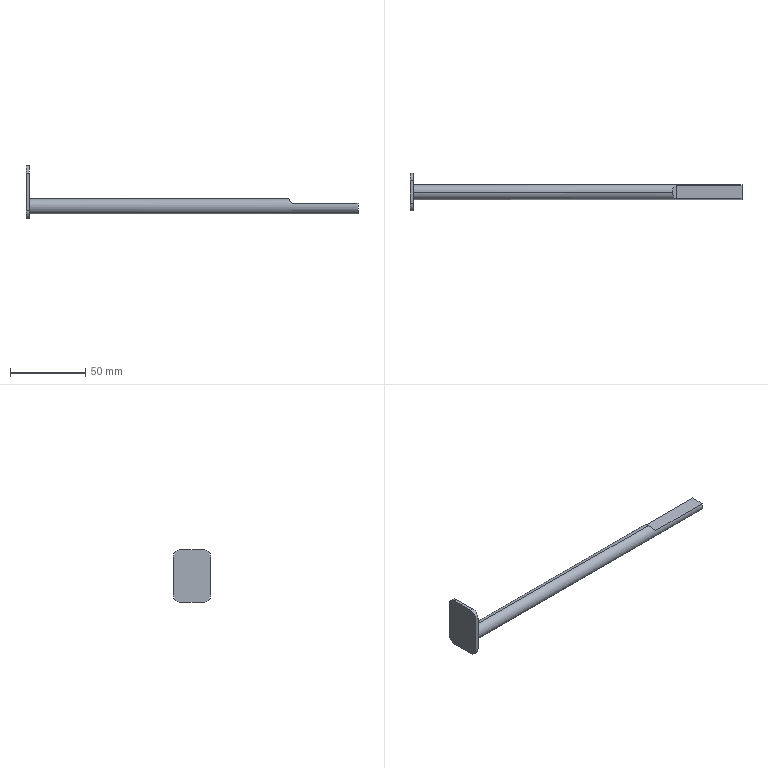Part | STEP file | 1 solid | 15 faces | box 220 x 25 x 35 mm | volume 17944 mm3 | plane 9 | cylinder 6 | commonest cylinder face diameters 10 x6
STEP:
#1=CARTESIAN_POINT('',(0.,0.,0.));
#2=DIRECTION('',(0.,0.,1.));
#3=DIRECTION('',(1.,0.,0.));
#4=AXIS2_PLACEMENT_3D('',#1,#2,#3);
#5=CARTESIAN_POINT('',(218.,45.399,13.874));
#6=VERTEX_POINT('',#5);
#7=CARTESIAN_POINT('',(218.,40.817,6.874));
#8=VERTEX_POINT('',#7);
#9=CARTESIAN_POINT('',(218.,40.817,11.874));
#10=DIRECTION('',(-1.,0.,0.));
#11=DIRECTION('',(0.,0.,1.));
#12=AXIS2_PLACEMENT_3D('',#9,#10,#11);
#13=CIRCLE('',#12,5.);
#14=CARTESIAN_POINT('',(218.,40.817,11.874));
#15=DIRECTION('',(-1.,0.,0.));
#16=DIRECTION('',(0.,0.,1.));
#17=AXIS2_PLACEMENT_3D('',#14,#15,#16);
#18=CYLINDRICAL_SURFACE('',#17,5.);
#19=CARTESIAN_POINT('',(0.,0.));
#20=DIRECTION('',(1.,0.));
#21=VECTOR('',#20,1.);
#22=LINE('',#19,#21);
#23=(GEOMETRIC_REPRESENTATION_CONTEXT(2)PARAMETRIC_REPRESENTATION_CONTEXT()REPRESENTATION_CONTEXT('',''));
#24=DEFINITIONAL_REPRESENTATION('',(#22),#23);
#25=PCURVE('',#18,#24);
#26=CARTESIAN_POINT('',(218.,40.817,11.874));
#27=DIRECTION('',(-1.,0.,0.));
#28=DIRECTION('',(0.,0.,1.));
#29=AXIS2_PLACEMENT_3D('',#26,#27,#28);
#30=PLANE('',#29);
#31=CARTESIAN_POINT('',(0.,0.));
#32=DIRECTION('',(1.,0.));
#33=AXIS2_PLACEMENT_2D('',#31,#32);
#34=CIRCLE('',#33,5.);
#35=(GEOMETRIC_REPRESENTATION_CONTEXT(2)PARAMETRIC_REPRESENTATION_CONTEXT()REPRESENTATION_CONTEXT('',''));
#36=DEFINITIONAL_REPRESENTATION('',(#34),#35);
#37=PCURVE('',#30,#36);
#38=SURFACE_CURVE('',#13,(#25,#37),.PCURVE_S1.);
#39=EDGE_CURVE('',#6,#8,#38,.T.);
#40=ORIENTED_EDGE('',*,*,#39,.T.);
#41=CARTESIAN_POINT('',(0.,40.817,6.874));
#42=VERTEX_POINT('',#41);
#43=CARTESIAN_POINT('',(218.,40.817,6.874));
#44=DIRECTION('',(-1.,0.,0.));
#45=VECTOR('',#44,1.);
#46=LINE('',#43,#45);
#47=CARTESIAN_POINT('',(3.142,0.));
#48=DIRECTION('',(0.,1.));
#49=VECTOR('',#48,1.);
#50=LINE('',#47,#49);
#51=(GEOMETRIC_REPRESENTATION_CONTEXT(2)PARAMETRIC_REPRESENTATION_CONTEXT()REPRESENTATION_CONTEXT('',''));
#52=DEFINITIONAL_REPRESENTATION('',(#50),#51);
#53=PCURVE('',#18,#52);
#54=CARTESIAN_POINT('',(218.,40.817,11.874));
#55=DIRECTION('',(-1.,0.,0.));
#56=DIRECTION('',(0.,0.,1.));
#57=AXIS2_PLACEMENT_3D('',#54,#55,#56);
#58=CYLINDRICAL_SURFACE('',#57,5.);
#59=CARTESIAN_POINT('',(3.142,0.));
#60=DIRECTION('',(0.,1.));
#61=VECTOR('',#60,1.);
#62=LINE('',#59,#61);
#63=(GEOMETRIC_REPRESENTATION_CONTEXT(2)PARAMETRIC_REPRESENTATION_CONTEXT()REPRESENTATION_CONTEXT('',''));
#64=DEFINITIONAL_REPRESENTATION('',(#62),#63);
#65=PCURVE('',#58,#64);
#66=SURFACE_CURVE('',#46,(#53,#65),.PCURVE_S1.);
#67=EDGE_CURVE('',#8,#42,#66,.T.);
#68=ORIENTED_EDGE('',*,*,#67,.T.);
#69=CARTESIAN_POINT('',(0.,40.817,16.874));
#70=VERTEX_POINT('',#69);
#71=CARTESIAN_POINT('',(0.,40.817,11.874));
#72=DIRECTION('',(1.,0.,0.));
#73=DIRECTION('',(0.,0.,-1.));
#74=AXIS2_PLACEMENT_3D('',#71,#72,#73);
#75=CIRCLE('',#74,5.);
#76=CARTESIAN_POINT('',(3.142,218.));
#77=DIRECTION('',(-1.,0.));
#78=VECTOR('',#77,1.);
#79=LINE('',#76,#78);
#80=(GEOMETRIC_REPRESENTATION_CONTEXT(2)PARAMETRIC_REPRESENTATION_CONTEXT()REPRESENTATION_CONTEXT('',''));
#81=DEFINITIONAL_REPRESENTATION('',(#79),#80);
#82=PCURVE('',#18,#81);
#83=CARTESIAN_POINT('',(0.,0.,0.));
#84=DIRECTION('',(1.,0.,0.));
#85=DIRECTION('',(0.,0.,-1.));
#86=AXIS2_PLACEMENT_3D('',#83,#84,#85);
#87=PLANE('',#86);
#88=CARTESIAN_POINT('',(-11.874,40.817));
#89=DIRECTION('',(1.,0.));
#90=AXIS2_PLACEMENT_2D('',#88,#89);
#91=CIRCLE('',#90,5.);
#92=(GEOMETRIC_REPRESENTATION_CONTEXT(2)PARAMETRIC_REPRESENTATION_CONTEXT()REPRESENTATION_CONTEXT('',''));
#93=DEFINITIONAL_REPRESENTATION('',(#91),#92);
#94=PCURVE('',#87,#93);
#95=SURFACE_CURVE('',#75,(#82,#94),.PCURVE_S1.);
#96=EDGE_CURVE('',#42,#70,#95,.T.);
#97=ORIENTED_EDGE('',*,*,#96,.T.);
#98=CARTESIAN_POINT('',(171.771,40.817,16.874));
#99=VERTEX_POINT('',#98);
#100=CARTESIAN_POINT('',(218.,40.817,16.874));
#101=DIRECTION('',(-1.,0.,0.));
#102=VECTOR('',#101,1.);
#103=LINE('',#100,#102);
#104=CARTESIAN_POINT('',(0.,0.));
#105=DIRECTION('',(0.,1.));
#106=VECTOR('',#105,1.);
#107=LINE('',#104,#106);
#108=(GEOMETRIC_REPRESENTATION_CONTEXT(2)PARAMETRIC_REPRESENTATION_CONTEXT()REPRESENTATION_CONTEXT('',''));
#109=DEFINITIONAL_REPRESENTATION('',(#107),#108);
#110=PCURVE('',#18,#109);
#111=CARTESIAN_POINT('',(6.283,0.));
#112=DIRECTION('',(0.,1.));
#113=VECTOR('',#112,1.);
#114=LINE('',#111,#113);
#115=(GEOMETRIC_REPRESENTATION_CONTEXT(2)PARAMETRIC_REPRESENTATION_CONTEXT()REPRESENTATION_CONTEXT('',''));
#116=DEFINITIONAL_REPRESENTATION('',(#114),#115);
#117=PCURVE('',#58,#116);
#118=SURFACE_CURVE('',#103,(#110,#117),.PCURVE_S1.);
#119=EDGE_CURVE('',#99,#70,#118,.T.);
#120=ORIENTED_EDGE('',*,*,#119,.F.);
#121=CARTESIAN_POINT('',(174.5,45.399,13.874));
#122=VERTEX_POINT('',#121);
#123=CARTESIAN_POINT('',(174.5,45.399,13.874));
#124=CARTESIAN_POINT('',(172.792,44.58,15.752));
#125=CARTESIAN_POINT('',(171.771,42.866,16.874));
#126=CARTESIAN_POINT('',(171.771,40.817,16.874));
#127=(BOUNDED_CURVE()B_SPLINE_CURVE(3,(#123,#124,#125,#126),.UNSPECIFIED.,.F.,.F.)B_SPLINE_CURVE_WITH_KNOTS((4,4),(5.124,6.283),.PIECEWISE_BEZIER_KNOTS.)CURVE()GEOMETRIC_REPRESENTATION_ITEM()RATIONAL_B_SPLINE_CURVE((1.,0.8911,0.8911,1.))REPRESENTATION_ITEM(''));
#128=CARTESIAN_POINT('',(1.159,43.5));
#129=CARTESIAN_POINT('',(1.143,43.569));
#130=CARTESIAN_POINT('',(1.109,43.707));
#131=CARTESIAN_POINT('',(1.058,43.912));
#132=CARTESIAN_POINT('',(1.007,44.113));
#133=CARTESIAN_POINT('',(0.9548,44.31));
#134=CARTESIAN_POINT('',(0.9022,44.501));
#135=CARTESIAN_POINT('',(0.8492,44.687));
#136=CARTESIAN_POINT('',(0.7957,44.865));
#137=CARTESIAN_POINT('',(0.742,45.035));
#138=CARTESIAN_POINT('',(0.688,45.196));
#139=CARTESIAN_POINT('',(0.6339,45.347));
#140=CARTESIAN_POINT('',(0.5796,45.488));
#141=CARTESIAN_POINT('',(0.5254,45.617));
#142=CARTESIAN_POINT('',(0.4713,45.735));
#143=CARTESIAN_POINT('',(0.4173,45.841));
#144=CARTESIAN_POINT('',(0.3635,45.934));
#145=CARTESIAN_POINT('',(0.3101,46.014));
#146=CARTESIAN_POINT('',(0.2571,46.081));
#147=CARTESIAN_POINT('',(0.2045,46.136));
#148=CARTESIAN_POINT('',(0.1524,46.178));
#149=CARTESIAN_POINT('',(0.1009,46.208));
#150=CARTESIAN_POINT('',(0.05004,46.225));
#151=CARTESIAN_POINT('',(0.0166,46.229));
#152=CARTESIAN_POINT('',(0.,46.229));
#153=B_SPLINE_CURVE_WITH_KNOTS('',3,(#128,#129,#130,#131,#132,#133,#134,#135,#136,#137,#138,#139,#140,#141,#142,#143,#144,#145,#146,#147,#148,#149,#150,#151,#152),.UNSPECIFIED.,.F.,.F.,(4,1,1,1,1,1,1,1,1,1,1,1,1,1,1,1,1,1,1,1,1,1,4),(5.124,5.177,5.229,5.282,5.335,5.387,5.44,5.493,5.545,5.598,5.651,5.704,5.756,5.809,5.862,5.914,5.967,6.02,6.072,6.125,6.178,6.23,6.283),.QUASI_UNIFORM_KNOTS.);
#154=(GEOMETRIC_REPRESENTATION_CONTEXT(2)PARAMETRIC_REPRESENTATION_CONTEXT()REPRESENTATION_CONTEXT('',''));
#155=DEFINITIONAL_REPRESENTATION('',(#153),#154);
#156=PCURVE('',#18,#155);
#157=CARTESIAN_POINT('',(174.5,53.317,13.874));
#158=DIRECTION('',(-0.7398,0.,-0.6729));
#159=DIRECTION('',(-0.6729,0.,0.7398));
#160=AXIS2_PLACEMENT_3D('',#157,#158,#159);
#161=PLANE('',#160);
#162=CARTESIAN_POINT('',(0.,-7.917));
#163=CARTESIAN_POINT('',(2.538,-8.737));
#164=CARTESIAN_POINT('',(4.055,-10.451));
#165=CARTESIAN_POINT('',(4.055,-12.5));
#166=(BOUNDED_CURVE()B_SPLINE_CURVE(3,(#162,#163,#164,#165),.UNSPECIFIED.,.F.,.F.)B_SPLINE_CURVE_WITH_KNOTS((4,4),(5.124,6.283),.PIECEWISE_BEZIER_KNOTS.)CURVE()GEOMETRIC_REPRESENTATION_ITEM()RATIONAL_B_SPLINE_CURVE((1.,0.8911,0.8911,1.))REPRESENTATION_ITEM(''));
#167=(GEOMETRIC_REPRESENTATION_CONTEXT(2)PARAMETRIC_REPRESENTATION_CONTEXT()REPRESENTATION_CONTEXT('',''));
#168=DEFINITIONAL_REPRESENTATION('',(#166),#167);
#169=PCURVE('',#161,#168);
#170=SURFACE_CURVE('',#127,(#156,#169),.PCURVE_S1.);
#171=EDGE_CURVE('',#122,#99,#170,.T.);
#172=ORIENTED_EDGE('',*,*,#171,.F.);
#173=CARTESIAN_POINT('',(218.,45.399,13.874));
#174=DIRECTION('',(-1.,0.,0.));
#175=VECTOR('',#174,1.);
#176=LINE('',#173,#175);
#177=CARTESIAN_POINT('',(1.159,0.));
#178=DIRECTION('',(0.,1.));
#179=VECTOR('',#178,1.);
#180=LINE('',#177,#179);
#181=(GEOMETRIC_REPRESENTATION_CONTEXT(2)PARAMETRIC_REPRESENTATION_CONTEXT()REPRESENTATION_CONTEXT('',''));
#182=DEFINITIONAL_REPRESENTATION('',(#180),#181);
#183=PCURVE('',#18,#182);
#184=CARTESIAN_POINT('',(174.5,21.274,13.874));
#185=DIRECTION('',(0.,0.,-1.));
#186=DIRECTION('',(-1.,0.,0.));
#187=AXIS2_PLACEMENT_3D('',#184,#185,#186);
#188=PLANE('',#187);
#189=CARTESIAN_POINT('',(-43.5,24.125));
#190=DIRECTION('',(1.,0.));
#191=VECTOR('',#190,1.);
#192=LINE('',#189,#191);
#193=(GEOMETRIC_REPRESENTATION_CONTEXT(2)PARAMETRIC_REPRESENTATION_CONTEXT()REPRESENTATION_CONTEXT('',''));
#194=DEFINITIONAL_REPRESENTATION('',(#192),#193);
#195=PCURVE('',#188,#194);
#196=SURFACE_CURVE('',#176,(#183,#195),.PCURVE_S1.);
#197=EDGE_CURVE('',#6,#122,#196,.T.);
#198=ORIENTED_EDGE('',*,*,#197,.F.);
#199=EDGE_LOOP('',(#40,#68,#97,#120,#172,#198));
#200=FACE_BOUND('',#199,.T.);
#201=ADVANCED_FACE('',(#200),#18,.T.);
#202=CARTESIAN_POINT('',(-2.,48.317,38.874));
#203=VERTEX_POINT('',#202);
#204=CARTESIAN_POINT('',(-2.,33.317,38.874));
#205=VERTEX_POINT('',#204);
#206=CARTESIAN_POINT('',(-2.,53.317,38.874));
#207=DIRECTION('',(0.,-1.,0.));
#208=VECTOR('',#207,1.);
#209=LINE('',#206,#208);
#210=CARTESIAN_POINT('',(-2.,53.317,38.874));
#211=DIRECTION('',(0.,0.,1.));
#212=DIRECTION('',(1.,0.,0.));
#213=AXIS2_PLACEMENT_3D('',#210,#211,#212);
#214=PLANE('',#213);
#215=CARTESIAN_POINT('',(0.,0.));
#216=DIRECTION('',(0.,-1.));
#217=VECTOR('',#216,1.);
#218=LINE('',#215,#217);
#219=(GEOMETRIC_REPRESENTATION_CONTEXT(2)PARAMETRIC_REPRESENTATION_CONTEXT()REPRESENTATION_CONTEXT('',''));
#220=DEFINITIONAL_REPRESENTATION('',(#218),#219);
#221=PCURVE('',#214,#220);
#222=CARTESIAN_POINT('',(-2.,0.,0.));
#223=DIRECTION('',(1.,0.,0.));
#224=DIRECTION('',(0.,0.,-1.));
#225=AXIS2_PLACEMENT_3D('',#222,#223,#224);
#226=PLANE('',#225);
#227=CARTESIAN_POINT('',(-38.874,53.317));
#228=DIRECTION('',(0.,-1.));
#229=VECTOR('',#228,1.);
#230=LINE('',#227,#229);
#231=(GEOMETRIC_REPRESENTATION_CONTEXT(2)PARAMETRIC_REPRESENTATION_CONTEXT()REPRESENTATION_CONTEXT('',''));
#232=DEFINITIONAL_REPRESENTATION('',(#230),#231);
#233=PCURVE('',#226,#232);
#234=SURFACE_CURVE('',#209,(#221,#233),.PCURVE_S1.);
#235=EDGE_CURVE('',#203,#205,#234,.T.);
#236=ORIENTED_EDGE('',*,*,#235,.T.);
#237=CARTESIAN_POINT('',(0.,33.317,38.874));
#238=VERTEX_POINT('',#237);
#239=CARTESIAN_POINT('',(-2.,33.317,38.874));
#240=DIRECTION('',(1.,0.,0.));
#241=VECTOR('',#240,1.);
#242=LINE('',#239,#241);
#243=CARTESIAN_POINT('',(0.,-20.));
#244=DIRECTION('',(1.,0.));
#245=VECTOR('',#244,1.);
#246=LINE('',#243,#245);
#247=(GEOMETRIC_REPRESENTATION_CONTEXT(2)PARAMETRIC_REPRESENTATION_CONTEXT()REPRESENTATION_CONTEXT('',''));
#248=DEFINITIONAL_REPRESENTATION('',(#246),#247);
#249=PCURVE('',#214,#248);
#250=CARTESIAN_POINT('',(-2.,33.317,33.874));
#251=DIRECTION('',(1.,0.,0.));
#252=DIRECTION('',(0.,0.,-1.));
#253=AXIS2_PLACEMENT_3D('',#250,#251,#252);
#254=CYLINDRICAL_SURFACE('',#253,5.);
#255=CARTESIAN_POINT('',(3.142,0.));
#256=DIRECTION('',(0.,1.));
#257=VECTOR('',#256,1.);
#258=LINE('',#255,#257);
#259=(GEOMETRIC_REPRESENTATION_CONTEXT(2)PARAMETRIC_REPRESENTATION_CONTEXT()REPRESENTATION_CONTEXT('',''));
#260=DEFINITIONAL_REPRESENTATION('',(#258),#259);
#261=PCURVE('',#254,#260);
#262=SURFACE_CURVE('',#242,(#249,#261),.PCURVE_S1.);
#263=EDGE_CURVE('',#205,#238,#262,.T.);
#264=ORIENTED_EDGE('',*,*,#263,.T.);
#265=CARTESIAN_POINT('',(0.,48.317,38.874));
#266=VERTEX_POINT('',#265);
#267=CARTESIAN_POINT('',(0.,53.317,38.874));
#268=DIRECTION('',(0.,-1.,0.));
#269=VECTOR('',#268,1.);
#270=LINE('',#267,#269);
#271=CARTESIAN_POINT('',(2.,0.));
#272=DIRECTION('',(0.,-1.));
#273=VECTOR('',#272,1.);
#274=LINE('',#271,#273);
#275=(GEOMETRIC_REPRESENTATION_CONTEXT(2)PARAMETRIC_REPRESENTATION_CONTEXT()REPRESENTATION_CONTEXT('',''));
#276=DEFINITIONAL_REPRESENTATION('',(#274),#275);
#277=PCURVE('',#214,#276);
#278=CARTESIAN_POINT('',(-38.874,53.317));
#279=DIRECTION('',(0.,-1.));
#280=VECTOR('',#279,1.);
#281=LINE('',#278,#280);
#282=(GEOMETRIC_REPRESENTATION_CONTEXT(2)PARAMETRIC_REPRESENTATION_CONTEXT()REPRESENTATION_CONTEXT('',''));
#283=DEFINITIONAL_REPRESENTATION('',(#281),#282);
#284=PCURVE('',#87,#283);
#285=SURFACE_CURVE('',#270,(#277,#284),.PCURVE_S1.);
#286=EDGE_CURVE('',#266,#238,#285,.T.);
#287=ORIENTED_EDGE('',*,*,#286,.F.);
#288=CARTESIAN_POINT('',(-2.,48.317,38.874));
#289=DIRECTION('',(-1.,0.,0.));
#290=VECTOR('',#289,1.);
#291=LINE('',#288,#290);
#292=CARTESIAN_POINT('',(0.,-5.));
#293=DIRECTION('',(-1.,0.));
#294=VECTOR('',#293,1.);
#295=LINE('',#292,#294);
#296=(GEOMETRIC_REPRESENTATION_CONTEXT(2)PARAMETRIC_REPRESENTATION_CONTEXT()REPRESENTATION_CONTEXT('',''));
#297=DEFINITIONAL_REPRESENTATION('',(#295),#296);
#298=PCURVE('',#214,#297);
#299=CARTESIAN_POINT('',(-2.,48.317,33.874));
#300=DIRECTION('',(1.,0.,0.));
#301=DIRECTION('',(0.,0.,-1.));
#302=AXIS2_PLACEMENT_3D('',#299,#300,#301);
#303=CYLINDRICAL_SURFACE('',#302,5.);
#304=CARTESIAN_POINT('',(3.142,0.));
#305=DIRECTION('',(0.,-1.));
#306=VECTOR('',#305,1.);
#307=LINE('',#304,#306);
#308=(GEOMETRIC_REPRESENTATION_CONTEXT(2)PARAMETRIC_REPRESENTATION_CONTEXT()REPRESENTATION_CONTEXT('',''));
#309=DEFINITIONAL_REPRESENTATION('',(#307),#308);
#310=PCURVE('',#303,#309);
#311=SURFACE_CURVE('',#291,(#298,#310),.PCURVE_S1.);
#312=EDGE_CURVE('',#266,#203,#311,.T.);
#313=ORIENTED_EDGE('',*,*,#312,.T.);
#314=EDGE_LOOP('',(#236,#264,#287,#313));
#315=FACE_BOUND('',#314,.T.);
#316=ADVANCED_FACE('',(#315),#214,.T.);
#317=CARTESIAN_POINT('',(0.,53.317,8.874));
#318=VERTEX_POINT('',#317);
#319=CARTESIAN_POINT('',(0.,53.317,33.874));
#320=VERTEX_POINT('',#319);
#321=CARTESIAN_POINT('',(0.,53.317,38.874));
#322=DIRECTION('',(0.,0.,1.));
#323=VECTOR('',#322,1.);
#324=LINE('',#321,#323);
#325=CARTESIAN_POINT('',(-2.,53.317,38.874));
#326=DIRECTION('',(0.,1.,0.));
#327=DIRECTION('',(0.,0.,1.));
#328=AXIS2_PLACEMENT_3D('',#325,#326,#327);
#329=PLANE('',#328);
#330=CARTESIAN_POINT('',(0.,2.));
#331=DIRECTION('',(1.,0.));
#332=VECTOR('',#331,1.);
#333=LINE('',#330,#332);
#334=(GEOMETRIC_REPRESENTATION_CONTEXT(2)PARAMETRIC_REPRESENTATION_CONTEXT()REPRESENTATION_CONTEXT('',''));
#335=DEFINITIONAL_REPRESENTATION('',(#333),#334);
#336=PCURVE('',#329,#335);
#337=CARTESIAN_POINT('',(-38.874,53.317));
#338=DIRECTION('',(-1.,0.));
#339=VECTOR('',#338,1.);
#340=LINE('',#337,#339);
#341=(GEOMETRIC_REPRESENTATION_CONTEXT(2)PARAMETRIC_REPRESENTATION_CONTEXT()REPRESENTATION_CONTEXT('',''));
#342=DEFINITIONAL_REPRESENTATION('',(#340),#341);
#343=PCURVE('',#87,#342);
#344=SURFACE_CURVE('',#324,(#336,#343),.PCURVE_S1.);
#345=EDGE_CURVE('',#318,#320,#344,.T.);
#346=ORIENTED_EDGE('',*,*,#345,.F.);
#347=CARTESIAN_POINT('',(-2.,53.317,8.874));
#348=VERTEX_POINT('',#347);
#349=CARTESIAN_POINT('',(-2.,53.317,8.874));
#350=DIRECTION('',(-1.,0.,0.));
#351=VECTOR('',#350,1.);
#352=LINE('',#349,#351);
#353=CARTESIAN_POINT('',(-30.,0.));
#354=DIRECTION('',(0.,-1.));
#355=VECTOR('',#354,1.);
#356=LINE('',#353,#355);
#357=(GEOMETRIC_REPRESENTATION_CONTEXT(2)PARAMETRIC_REPRESENTATION_CONTEXT()REPRESENTATION_CONTEXT('',''));
#358=DEFINITIONAL_REPRESENTATION('',(#356),#357);
#359=PCURVE('',#329,#358);
#360=CARTESIAN_POINT('',(-2.,48.317,8.874));
#361=DIRECTION('',(1.,0.,0.));
#362=DIRECTION('',(0.,0.,-1.));
#363=AXIS2_PLACEMENT_3D('',#360,#361,#362);
#364=CYLINDRICAL_SURFACE('',#363,5.);
#365=CARTESIAN_POINT('',(1.571,0.));
#366=DIRECTION('',(0.,-1.));
#367=VECTOR('',#366,1.);
#368=LINE('',#365,#367);
#369=(GEOMETRIC_REPRESENTATION_CONTEXT(2)PARAMETRIC_REPRESENTATION_CONTEXT()REPRESENTATION_CONTEXT('',''));
#370=DEFINITIONAL_REPRESENTATION('',(#368),#369);
#371=PCURVE('',#364,#370);
#372=SURFACE_CURVE('',#352,(#359,#371),.PCURVE_S1.);
#373=EDGE_CURVE('',#318,#348,#372,.T.);
#374=ORIENTED_EDGE('',*,*,#373,.T.);
#375=CARTESIAN_POINT('',(-2.,53.317,33.874));
#376=VERTEX_POINT('',#375);
#377=CARTESIAN_POINT('',(-2.,53.317,38.874));
#378=DIRECTION('',(0.,0.,1.));
#379=VECTOR('',#378,1.);
#380=LINE('',#377,#379);
#381=CARTESIAN_POINT('',(0.,0.));
#382=DIRECTION('',(1.,0.));
#383=VECTOR('',#382,1.);
#384=LINE('',#381,#383);
#385=(GEOMETRIC_REPRESENTATION_CONTEXT(2)PARAMETRIC_REPRESENTATION_CONTEXT()REPRESENTATION_CONTEXT('',''));
#386=DEFINITIONAL_REPRESENTATION('',(#384),#385);
#387=PCURVE('',#329,#386);
#388=CARTESIAN_POINT('',(-38.874,53.317));
#389=DIRECTION('',(-1.,0.));
#390=VECTOR('',#389,1.);
#391=LINE('',#388,#390);
#392=(GEOMETRIC_REPRESENTATION_CONTEXT(2)PARAMETRIC_REPRESENTATION_CONTEXT()REPRESENTATION_CONTEXT('',''));
#393=DEFINITIONAL_REPRESENTATION('',(#391),#392);
#394=PCURVE('',#226,#393);
#395=SURFACE_CURVE('',#380,(#387,#394),.PCURVE_S1.);
#396=EDGE_CURVE('',#348,#376,#395,.T.);
#397=ORIENTED_EDGE('',*,*,#396,.T.);
#398=CARTESIAN_POINT('',(-2.,53.317,33.874));
#399=DIRECTION('',(1.,0.,0.));
#400=VECTOR('',#399,1.);
#401=LINE('',#398,#400);
#402=CARTESIAN_POINT('',(-5.,0.));
#403=DIRECTION('',(0.,1.));
#404=VECTOR('',#403,1.);
#405=LINE('',#402,#404);
#406=(GEOMETRIC_REPRESENTATION_CONTEXT(2)PARAMETRIC_REPRESENTATION_CONTEXT()REPRESENTATION_CONTEXT('',''));
#407=DEFINITIONAL_REPRESENTATION('',(#405),#406);
#408=PCURVE('',#329,#407);
#409=CARTESIAN_POINT('',(1.571,0.));
#410=DIRECTION('',(0.,1.));
#411=VECTOR('',#410,1.);
#412=LINE('',#409,#411);
#413=(GEOMETRIC_REPRESENTATION_CONTEXT(2)PARAMETRIC_REPRESENTATION_CONTEXT()REPRESENTATION_CONTEXT('',''));
#414=DEFINITIONAL_REPRESENTATION('',(#412),#413);
#415=PCURVE('',#303,#414);
#416=SURFACE_CURVE('',#401,(#408,#415),.PCURVE_S1.);
#417=EDGE_CURVE('',#376,#320,#416,.T.);
#418=ORIENTED_EDGE('',*,*,#417,.T.);
#419=EDGE_LOOP('',(#346,#374,#397,#418));
#420=FACE_BOUND('',#419,.T.);
#421=ADVANCED_FACE('',(#420),#329,.T.);
#422=CARTESIAN_POINT('',(0.,33.317,3.874));
#423=VERTEX_POINT('',#422);
#424=CARTESIAN_POINT('',(0.,48.317,3.874));
#425=VERTEX_POINT('',#424);
#426=CARTESIAN_POINT('',(0.,53.317,3.874));
#427=DIRECTION('',(0.,1.,0.));
#428=VECTOR('',#427,1.);
#429=LINE('',#426,#428);
#430=CARTESIAN_POINT('',(-2.,53.317,3.874));
#431=DIRECTION('',(0.,0.,-1.));
#432=DIRECTION('',(-1.,0.,0.));
#433=AXIS2_PLACEMENT_3D('',#430,#431,#432);
#434=PLANE('',#433);
#435=CARTESIAN_POINT('',(-2.,0.));
#436=DIRECTION('',(0.,1.));
#437=VECTOR('',#436,1.);
#438=LINE('',#435,#437);
#439=(GEOMETRIC_REPRESENTATION_CONTEXT(2)PARAMETRIC_REPRESENTATION_CONTEXT()REPRESENTATION_CONTEXT('',''));
#440=DEFINITIONAL_REPRESENTATION('',(#438),#439);
#441=PCURVE('',#434,#440);
#442=CARTESIAN_POINT('',(-3.874,53.317));
#443=DIRECTION('',(0.,1.));
#444=VECTOR('',#443,1.);
#445=LINE('',#442,#444);
#446=(GEOMETRIC_REPRESENTATION_CONTEXT(2)PARAMETRIC_REPRESENTATION_CONTEXT()REPRESENTATION_CONTEXT('',''));
#447=DEFINITIONAL_REPRESENTATION('',(#445),#446);
#448=PCURVE('',#87,#447);
#449=SURFACE_CURVE('',#429,(#441,#448),.PCURVE_S1.);
#450=EDGE_CURVE('',#423,#425,#449,.T.);
#451=ORIENTED_EDGE('',*,*,#450,.F.);
#452=CARTESIAN_POINT('',(-2.,33.317,3.874));
#453=VERTEX_POINT('',#452);
#454=CARTESIAN_POINT('',(-2.,33.317,3.874));
#455=DIRECTION('',(-1.,0.,0.));
#456=VECTOR('',#455,1.);
#457=LINE('',#454,#456);
#458=CARTESIAN_POINT('',(0.,-20.));
#459=DIRECTION('',(1.,0.));
#460=VECTOR('',#459,1.);
#461=LINE('',#458,#460);
#462=(GEOMETRIC_REPRESENTATION_CONTEXT(2)PARAMETRIC_REPRESENTATION_CONTEXT()REPRESENTATION_CONTEXT('',''));
#463=DEFINITIONAL_REPRESENTATION('',(#461),#462);
#464=PCURVE('',#434,#463);
#465=CARTESIAN_POINT('',(-2.,33.317,8.874));
#466=DIRECTION('',(1.,0.,0.));
#467=DIRECTION('',(0.,0.,-1.));
#468=AXIS2_PLACEMENT_3D('',#465,#466,#467);
#469=CYLINDRICAL_SURFACE('',#468,5.);
#470=CARTESIAN_POINT('',(6.283,0.));
#471=DIRECTION('',(0.,-1.));
#472=VECTOR('',#471,1.);
#473=LINE('',#470,#472);
#474=(GEOMETRIC_REPRESENTATION_CONTEXT(2)PARAMETRIC_REPRESENTATION_CONTEXT()REPRESENTATION_CONTEXT('',''));
#475=DEFINITIONAL_REPRESENTATION('',(#473),#474);
#476=PCURVE('',#469,#475);
#477=SURFACE_CURVE('',#457,(#464,#476),.PCURVE_S1.);
#478=EDGE_CURVE('',#423,#453,#477,.T.);
#479=ORIENTED_EDGE('',*,*,#478,.T.);
#480=CARTESIAN_POINT('',(-2.,48.317,3.874));
#481=VERTEX_POINT('',#480);
#482=CARTESIAN_POINT('',(-2.,53.317,3.874));
#483=DIRECTION('',(0.,1.,0.));
#484=VECTOR('',#483,1.);
#485=LINE('',#482,#484);
#486=CARTESIAN_POINT('',(0.,0.));
#487=DIRECTION('',(0.,1.));
#488=VECTOR('',#487,1.);
#489=LINE('',#486,#488);
#490=(GEOMETRIC_REPRESENTATION_CONTEXT(2)PARAMETRIC_REPRESENTATION_CONTEXT()REPRESENTATION_CONTEXT('',''));
#491=DEFINITIONAL_REPRESENTATION('',(#489),#490);
#492=PCURVE('',#434,#491);
#493=CARTESIAN_POINT('',(-3.874,53.317));
#494=DIRECTION('',(0.,1.));
#495=VECTOR('',#494,1.);
#496=LINE('',#493,#495);
#497=(GEOMETRIC_REPRESENTATION_CONTEXT(2)PARAMETRIC_REPRESENTATION_CONTEXT()REPRESENTATION_CONTEXT('',''));
#498=DEFINITIONAL_REPRESENTATION('',(#496),#497);
#499=PCURVE('',#226,#498);
#500=SURFACE_CURVE('',#485,(#492,#499),.PCURVE_S1.);
#501=EDGE_CURVE('',#453,#481,#500,.T.);
#502=ORIENTED_EDGE('',*,*,#501,.T.);
#503=CARTESIAN_POINT('',(-2.,48.317,3.874));
#504=DIRECTION('',(1.,0.,0.));
#505=VECTOR('',#504,1.);
#506=LINE('',#503,#505);
#507=CARTESIAN_POINT('',(0.,-5.));
#508=DIRECTION('',(-1.,0.));
#509=VECTOR('',#508,1.);
#510=LINE('',#507,#509);
#511=(GEOMETRIC_REPRESENTATION_CONTEXT(2)PARAMETRIC_REPRESENTATION_CONTEXT()REPRESENTATION_CONTEXT('',''));
#512=DEFINITIONAL_REPRESENTATION('',(#510),#511);
#513=PCURVE('',#434,#512);
#514=CARTESIAN_POINT('',(0.,0.));
#515=DIRECTION('',(0.,1.));
#516=VECTOR('',#515,1.);
#517=LINE('',#514,#516);
#518=(GEOMETRIC_REPRESENTATION_CONTEXT(2)PARAMETRIC_REPRESENTATION_CONTEXT()REPRESENTATION_CONTEXT('',''));
#519=DEFINITIONAL_REPRESENTATION('',(#517),#518);
#520=PCURVE('',#364,#519);
#521=SURFACE_CURVE('',#506,(#513,#520),.PCURVE_S1.);
#522=EDGE_CURVE('',#481,#425,#521,.T.);
#523=ORIENTED_EDGE('',*,*,#522,.T.);
#524=EDGE_LOOP('',(#451,#479,#502,#523));
#525=FACE_BOUND('',#524,.T.);
#526=ADVANCED_FACE('',(#525),#434,.T.);
#527=CARTESIAN_POINT('',(-2.,28.317,33.874));
#528=VERTEX_POINT('',#527);
#529=CARTESIAN_POINT('',(-2.,28.317,8.874));
#530=VERTEX_POINT('',#529);
#531=CARTESIAN_POINT('',(-2.,28.317,38.874));
#532=DIRECTION('',(0.,0.,-1.));
#533=VECTOR('',#532,1.);
#534=LINE('',#531,#533);
#535=CARTESIAN_POINT('',(-2.,28.317,38.874));
#536=DIRECTION('',(0.,-1.,0.));
#537=DIRECTION('',(0.,0.,-1.));
#538=AXIS2_PLACEMENT_3D('',#535,#536,#537);
#539=PLANE('',#538);
#540=CARTESIAN_POINT('',(0.,0.));
#541=DIRECTION('',(1.,0.));
#542=VECTOR('',#541,1.);
#543=LINE('',#540,#542);
#544=(GEOMETRIC_REPRESENTATION_CONTEXT(2)PARAMETRIC_REPRESENTATION_CONTEXT()REPRESENTATION_CONTEXT('',''));
#545=DEFINITIONAL_REPRESENTATION('',(#543),#544);
#546=PCURVE('',#539,#545);
#547=CARTESIAN_POINT('',(-38.874,28.317));
#548=DIRECTION('',(1.,0.));
#549=VECTOR('',#548,1.);
#550=LINE('',#547,#549);
#551=(GEOMETRIC_REPRESENTATION_CONTEXT(2)PARAMETRIC_REPRESENTATION_CONTEXT()REPRESENTATION_CONTEXT('',''));
#552=DEFINITIONAL_REPRESENTATION('',(#550),#551);
#553=PCURVE('',#226,#552);
#554=SURFACE_CURVE('',#534,(#546,#553),.PCURVE_S1.);
#555=EDGE_CURVE('',#528,#530,#554,.T.);
#556=ORIENTED_EDGE('',*,*,#555,.T.);
#557=CARTESIAN_POINT('',(0.,28.317,8.874));
#558=VERTEX_POINT('',#557);
#559=CARTESIAN_POINT('',(-2.,28.317,8.874));
#560=DIRECTION('',(1.,0.,0.));
#561=VECTOR('',#560,1.);
#562=LINE('',#559,#561);
#563=CARTESIAN_POINT('',(30.,0.));
#564=DIRECTION('',(0.,1.));
#565=VECTOR('',#564,1.);
#566=LINE('',#563,#565);
#567=(GEOMETRIC_REPRESENTATION_CONTEXT(2)PARAMETRIC_REPRESENTATION_CONTEXT()REPRESENTATION_CONTEXT('',''));
#568=DEFINITIONAL_REPRESENTATION('',(#566),#567);
#569=PCURVE('',#539,#568);
#570=CARTESIAN_POINT('',(4.712,0.));
#571=DIRECTION('',(0.,1.));
#572=VECTOR('',#571,1.);
#573=LINE('',#570,#572);
#574=(GEOMETRIC_REPRESENTATION_CONTEXT(2)PARAMETRIC_REPRESENTATION_CONTEXT()REPRESENTATION_CONTEXT('',''));
#575=DEFINITIONAL_REPRESENTATION('',(#573),#574);
#576=PCURVE('',#469,#575);
#577=SURFACE_CURVE('',#562,(#569,#576),.PCURVE_S1.);
#578=EDGE_CURVE('',#530,#558,#577,.T.);
#579=ORIENTED_EDGE('',*,*,#578,.T.);
#580=CARTESIAN_POINT('',(0.,28.317,33.874));
#581=VERTEX_POINT('',#580);
#582=CARTESIAN_POINT('',(0.,28.317,38.874));
#583=DIRECTION('',(0.,0.,-1.));
#584=VECTOR('',#583,1.);
#585=LINE('',#582,#584);
#586=CARTESIAN_POINT('',(0.,2.));
#587=DIRECTION('',(1.,0.));
#588=VECTOR('',#587,1.);
#589=LINE('',#586,#588);
#590=(GEOMETRIC_REPRESENTATION_CONTEXT(2)PARAMETRIC_REPRESENTATION_CONTEXT()REPRESENTATION_CONTEXT('',''));
#591=DEFINITIONAL_REPRESENTATION('',(#589),#590);
#592=PCURVE('',#539,#591);
#593=CARTESIAN_POINT('',(-38.874,28.317));
#594=DIRECTION('',(1.,0.));
#595=VECTOR('',#594,1.);
#596=LINE('',#593,#595);
#597=(GEOMETRIC_REPRESENTATION_CONTEXT(2)PARAMETRIC_REPRESENTATION_CONTEXT()REPRESENTATION_CONTEXT('',''));
#598=DEFINITIONAL_REPRESENTATION('',(#596),#597);
#599=PCURVE('',#87,#598);
#600=SURFACE_CURVE('',#585,(#592,#599),.PCURVE_S1.);
#601=EDGE_CURVE('',#581,#558,#600,.T.);
#602=ORIENTED_EDGE('',*,*,#601,.F.);
#603=CARTESIAN_POINT('',(-2.,28.317,33.874));
#604=DIRECTION('',(-1.,0.,0.));
#605=VECTOR('',#604,1.);
#606=LINE('',#603,#605);
#607=CARTESIAN_POINT('',(5.,0.));
#608=DIRECTION('',(0.,-1.));
#609=VECTOR('',#608,1.);
#610=LINE('',#607,#609);
#611=(GEOMETRIC_REPRESENTATION_CONTEXT(2)PARAMETRIC_REPRESENTATION_CONTEXT()REPRESENTATION_CONTEXT('',''));
#612=DEFINITIONAL_REPRESENTATION('',(#610),#611);
#613=PCURVE('',#539,#612);
#614=CARTESIAN_POINT('',(4.712,0.));
#615=DIRECTION('',(0.,-1.));
#616=VECTOR('',#615,1.);
#617=LINE('',#614,#616);
#618=(GEOMETRIC_REPRESENTATION_CONTEXT(2)PARAMETRIC_REPRESENTATION_CONTEXT()REPRESENTATION_CONTEXT('',''));
#619=DEFINITIONAL_REPRESENTATION('',(#617),#618);
#620=PCURVE('',#254,#619);
#621=SURFACE_CURVE('',#606,(#613,#620),.PCURVE_S1.);
#622=EDGE_CURVE('',#581,#528,#621,.T.);
#623=ORIENTED_EDGE('',*,*,#622,.T.);
#624=EDGE_LOOP('',(#556,#579,#602,#623));
#625=FACE_BOUND('',#624,.T.);
#626=ADVANCED_FACE('',(#625),#539,.T.);
#627=ORIENTED_EDGE('',*,*,#501,.F.);
#628=CARTESIAN_POINT('',(-2.,33.317,8.874));
#629=DIRECTION('',(-1.,0.,0.));
#630=DIRECTION('',(0.,0.,-1.));
#631=AXIS2_PLACEMENT_3D('',#628,#629,#630);
#632=CIRCLE('',#631,5.);
#633=CARTESIAN_POINT('',(-3.874,33.317));
#634=CARTESIAN_POINT('',(-3.874,24.656));
#635=CARTESIAN_POINT('',(-11.374,28.987));
#636=CARTESIAN_POINT('',(-18.874,33.317));
#637=CARTESIAN_POINT('',(-11.374,37.647));
#638=CARTESIAN_POINT('',(-3.874,41.977));
#639=CARTESIAN_POINT('',(-3.874,33.317));
#640=(BOUNDED_CURVE()B_SPLINE_CURVE(2,(#633,#634,#635,#636,#637,#638,#639),.UNSPECIFIED.,.T.,.F.)B_SPLINE_CURVE_WITH_KNOTS((1,2,2,2,2,1),(-2.094,0.,2.094,4.189,6.283,8.378),.UNSPECIFIED.)CURVE()GEOMETRIC_REPRESENTATION_ITEM()RATIONAL_B_SPLINE_CURVE((1.,0.5,1.,0.5,1.,0.5,1.))REPRESENTATION_ITEM(''));
#641=(GEOMETRIC_REPRESENTATION_CONTEXT(2)PARAMETRIC_REPRESENTATION_CONTEXT()REPRESENTATION_CONTEXT('',''));
#642=DEFINITIONAL_REPRESENTATION('',(#640),#641);
#643=PCURVE('',#226,#642);
#644=CARTESIAN_POINT('',(6.283,0.));
#645=DIRECTION('',(-1.,0.));
#646=VECTOR('',#645,1.);
#647=LINE('',#644,#646);
#648=(GEOMETRIC_REPRESENTATION_CONTEXT(2)PARAMETRIC_REPRESENTATION_CONTEXT()REPRESENTATION_CONTEXT('',''));
#649=DEFINITIONAL_REPRESENTATION('',(#647),#648);
#650=PCURVE('',#469,#649);
#651=SURFACE_CURVE('',#632,(#643,#650),.PCURVE_S1.);
#652=EDGE_CURVE('',#453,#530,#651,.T.);
#653=ORIENTED_EDGE('',*,*,#652,.T.);
#654=ORIENTED_EDGE('',*,*,#555,.F.);
#655=CARTESIAN_POINT('',(-2.,33.317,33.874));
#656=DIRECTION('',(-1.,0.,0.));
#657=DIRECTION('',(0.,0.,-1.));
#658=AXIS2_PLACEMENT_3D('',#655,#656,#657);
#659=CIRCLE('',#658,5.);
#660=CARTESIAN_POINT('',(-28.874,33.317));
#661=CARTESIAN_POINT('',(-28.874,24.656));
#662=CARTESIAN_POINT('',(-36.374,28.987));
#663=CARTESIAN_POINT('',(-43.874,33.317));
#664=CARTESIAN_POINT('',(-36.374,37.647));
#665=CARTESIAN_POINT('',(-28.874,41.977));
#666=CARTESIAN_POINT('',(-28.874,33.317));
#667=(BOUNDED_CURVE()B_SPLINE_CURVE(2,(#660,#661,#662,#663,#664,#665,#666),.UNSPECIFIED.,.T.,.F.)B_SPLINE_CURVE_WITH_KNOTS((1,2,2,2,2,1),(-2.094,0.,2.094,4.189,6.283,8.378),.UNSPECIFIED.)CURVE()GEOMETRIC_REPRESENTATION_ITEM()RATIONAL_B_SPLINE_CURVE((1.,0.5,1.,0.5,1.,0.5,1.))REPRESENTATION_ITEM(''));
#668=(GEOMETRIC_REPRESENTATION_CONTEXT(2)PARAMETRIC_REPRESENTATION_CONTEXT()REPRESENTATION_CONTEXT('',''));
#669=DEFINITIONAL_REPRESENTATION('',(#667),#668);
#670=PCURVE('',#226,#669);
#671=CARTESIAN_POINT('',(6.283,0.));
#672=DIRECTION('',(-1.,0.));
#673=VECTOR('',#672,1.);
#674=LINE('',#671,#673);
#675=(GEOMETRIC_REPRESENTATION_CONTEXT(2)PARAMETRIC_REPRESENTATION_CONTEXT()REPRESENTATION_CONTEXT('',''));
#676=DEFINITIONAL_REPRESENTATION('',(#674),#675);
#677=PCURVE('',#254,#676);
#678=SURFACE_CURVE('',#659,(#670,#677),.PCURVE_S1.);
#679=EDGE_CURVE('',#528,#205,#678,.T.);
#680=ORIENTED_EDGE('',*,*,#679,.T.);
#681=ORIENTED_EDGE('',*,*,#235,.F.);
#682=CARTESIAN_POINT('',(-2.,48.317,33.874));
#683=DIRECTION('',(-1.,0.,0.));
#684=DIRECTION('',(0.,0.,-1.));
#685=AXIS2_PLACEMENT_3D('',#682,#683,#684);
#686=CIRCLE('',#685,5.);
#687=CARTESIAN_POINT('',(-28.874,48.317));
#688=CARTESIAN_POINT('',(-28.874,39.656));
#689=CARTESIAN_POINT('',(-36.374,43.987));
#690=CARTESIAN_POINT('',(-43.874,48.317));
#691=CARTESIAN_POINT('',(-36.374,52.647));
#692=CARTESIAN_POINT('',(-28.874,56.977));
#693=CARTESIAN_POINT('',(-28.874,48.317));
#694=(BOUNDED_CURVE()B_SPLINE_CURVE(2,(#687,#688,#689,#690,#691,#692,#693),.UNSPECIFIED.,.T.,.F.)B_SPLINE_CURVE_WITH_KNOTS((1,2,2,2,2,1),(-2.094,0.,2.094,4.189,6.283,8.378),.UNSPECIFIED.)CURVE()GEOMETRIC_REPRESENTATION_ITEM()RATIONAL_B_SPLINE_CURVE((1.,0.5,1.,0.5,1.,0.5,1.))REPRESENTATION_ITEM(''));
#695=(GEOMETRIC_REPRESENTATION_CONTEXT(2)PARAMETRIC_REPRESENTATION_CONTEXT()REPRESENTATION_CONTEXT('',''));
#696=DEFINITIONAL_REPRESENTATION('',(#694),#695);
#697=PCURVE('',#226,#696);
#698=CARTESIAN_POINT('',(6.283,0.));
#699=DIRECTION('',(-1.,0.));
#700=VECTOR('',#699,1.);
#701=LINE('',#698,#700);
#702=(GEOMETRIC_REPRESENTATION_CONTEXT(2)PARAMETRIC_REPRESENTATION_CONTEXT()REPRESENTATION_CONTEXT('',''));
#703=DEFINITIONAL_REPRESENTATION('',(#701),#702);
#704=PCURVE('',#303,#703);
#705=SURFACE_CURVE('',#686,(#697,#704),.PCURVE_S1.);
#706=EDGE_CURVE('',#203,#376,#705,.T.);
#707=ORIENTED_EDGE('',*,*,#706,.T.);
#708=ORIENTED_EDGE('',*,*,#396,.F.);
#709=CARTESIAN_POINT('',(-2.,48.317,8.874));
#710=DIRECTION('',(-1.,0.,0.));
#711=DIRECTION('',(0.,0.,-1.));
#712=AXIS2_PLACEMENT_3D('',#709,#710,#711);
#713=CIRCLE('',#712,5.);
#714=CARTESIAN_POINT('',(-3.874,48.317));
#715=CARTESIAN_POINT('',(-3.874,39.656));
#716=CARTESIAN_POINT('',(-11.374,43.987));
#717=CARTESIAN_POINT('',(-18.874,48.317));
#718=CARTESIAN_POINT('',(-11.374,52.647));
#719=CARTESIAN_POINT('',(-3.874,56.977));
#720=CARTESIAN_POINT('',(-3.874,48.317));
#721=(BOUNDED_CURVE()B_SPLINE_CURVE(2,(#714,#715,#716,#717,#718,#719,#720),.UNSPECIFIED.,.T.,.F.)B_SPLINE_CURVE_WITH_KNOTS((1,2,2,2,2,1),(-2.094,0.,2.094,4.189,6.283,8.378),.UNSPECIFIED.)CURVE()GEOMETRIC_REPRESENTATION_ITEM()RATIONAL_B_SPLINE_CURVE((1.,0.5,1.,0.5,1.,0.5,1.))REPRESENTATION_ITEM(''));
#722=(GEOMETRIC_REPRESENTATION_CONTEXT(2)PARAMETRIC_REPRESENTATION_CONTEXT()REPRESENTATION_CONTEXT('',''));
#723=DEFINITIONAL_REPRESENTATION('',(#721),#722);
#724=PCURVE('',#226,#723);
#725=CARTESIAN_POINT('',(6.283,0.));
#726=DIRECTION('',(-1.,0.));
#727=VECTOR('',#726,1.);
#728=LINE('',#725,#727);
#729=(GEOMETRIC_REPRESENTATION_CONTEXT(2)PARAMETRIC_REPRESENTATION_CONTEXT()REPRESENTATION_CONTEXT('',''));
#730=DEFINITIONAL_REPRESENTATION('',(#728),#729);
#731=PCURVE('',#364,#730);
#732=SURFACE_CURVE('',#713,(#724,#731),.PCURVE_S1.);
#733=EDGE_CURVE('',#348,#481,#732,.T.);
#734=ORIENTED_EDGE('',*,*,#733,.T.);
#735=EDGE_LOOP('',(#627,#653,#654,#680,#681,#707,#708,#734));
#736=FACE_BOUND('',#735,.T.);
#737=ADVANCED_FACE('',(#736),#226,.F.);
#738=CARTESIAN_POINT('',(0.,40.817,11.874));
#739=DIRECTION('',(1.,0.,0.));
#740=DIRECTION('',(0.,0.,-1.));
#741=AXIS2_PLACEMENT_3D('',#738,#739,#740);
#742=CIRCLE('',#741,5.);
#743=CARTESIAN_POINT('',(-11.874,40.817));
#744=DIRECTION('',(1.,0.));
#745=AXIS2_PLACEMENT_2D('',#743,#744);
#746=CIRCLE('',#745,5.);
#747=(GEOMETRIC_REPRESENTATION_CONTEXT(2)PARAMETRIC_REPRESENTATION_CONTEXT()REPRESENTATION_CONTEXT('',''));
#748=DEFINITIONAL_REPRESENTATION('',(#746),#747);
#749=PCURVE('',#87,#748);
#750=CARTESIAN_POINT('',(9.425,218.));
#751=DIRECTION('',(-1.,0.));
#752=VECTOR('',#751,1.);
#753=LINE('',#750,#752);
#754=(GEOMETRIC_REPRESENTATION_CONTEXT(2)PARAMETRIC_REPRESENTATION_CONTEXT()REPRESENTATION_CONTEXT('',''));
#755=DEFINITIONAL_REPRESENTATION('',(#753),#754);
#756=PCURVE('',#58,#755);
#757=SURFACE_CURVE('',#742,(#749,#756),.PCURVE_S1.);
#758=EDGE_CURVE('',#70,#42,#757,.T.);
#759=ORIENTED_EDGE('',*,*,#758,.F.);
#760=ORIENTED_EDGE('',*,*,#96,.F.);
#761=EDGE_LOOP('',(#759,#760));
#762=FACE_BOUND('',#761,.T.);
#763=ORIENTED_EDGE('',*,*,#601,.T.);
#764=CARTESIAN_POINT('',(0.,33.317,8.874));
#765=DIRECTION('',(1.,0.,0.));
#766=DIRECTION('',(0.,0.,-1.));
#767=AXIS2_PLACEMENT_3D('',#764,#765,#766);
#768=CIRCLE('',#767,5.);
#769=CARTESIAN_POINT('',(-8.874,33.317));
#770=DIRECTION('',(1.,0.));
#771=AXIS2_PLACEMENT_2D('',#769,#770);
#772=CIRCLE('',#771,5.);
#773=(GEOMETRIC_REPRESENTATION_CONTEXT(2)PARAMETRIC_REPRESENTATION_CONTEXT()REPRESENTATION_CONTEXT('',''));
#774=DEFINITIONAL_REPRESENTATION('',(#772),#773);
#775=PCURVE('',#87,#774);
#776=CARTESIAN_POINT('',(0.,2.));
#777=DIRECTION('',(1.,0.));
#778=VECTOR('',#777,1.);
#779=LINE('',#776,#778);
#780=(GEOMETRIC_REPRESENTATION_CONTEXT(2)PARAMETRIC_REPRESENTATION_CONTEXT()REPRESENTATION_CONTEXT('',''));
#781=DEFINITIONAL_REPRESENTATION('',(#779),#780);
#782=PCURVE('',#469,#781);
#783=SURFACE_CURVE('',#768,(#775,#782),.PCURVE_S1.);
#784=EDGE_CURVE('',#558,#423,#783,.T.);
#785=ORIENTED_EDGE('',*,*,#784,.T.);
#786=ORIENTED_EDGE('',*,*,#450,.T.);
#787=CARTESIAN_POINT('',(0.,48.317,8.874));
#788=DIRECTION('',(1.,0.,0.));
#789=DIRECTION('',(0.,0.,-1.));
#790=AXIS2_PLACEMENT_3D('',#787,#788,#789);
#791=CIRCLE('',#790,5.);
#792=CARTESIAN_POINT('',(-8.874,48.317));
#793=DIRECTION('',(1.,0.));
#794=AXIS2_PLACEMENT_2D('',#792,#793);
#795=CIRCLE('',#794,5.);
#796=(GEOMETRIC_REPRESENTATION_CONTEXT(2)PARAMETRIC_REPRESENTATION_CONTEXT()REPRESENTATION_CONTEXT('',''));
#797=DEFINITIONAL_REPRESENTATION('',(#795),#796);
#798=PCURVE('',#87,#797);
#799=CARTESIAN_POINT('',(0.,2.));
#800=DIRECTION('',(1.,0.));
#801=VECTOR('',#800,1.);
#802=LINE('',#799,#801);
#803=(GEOMETRIC_REPRESENTATION_CONTEXT(2)PARAMETRIC_REPRESENTATION_CONTEXT()REPRESENTATION_CONTEXT('',''));
#804=DEFINITIONAL_REPRESENTATION('',(#802),#803);
#805=PCURVE('',#364,#804);
#806=SURFACE_CURVE('',#791,(#798,#805),.PCURVE_S1.);
#807=EDGE_CURVE('',#425,#318,#806,.T.);
#808=ORIENTED_EDGE('',*,*,#807,.T.);
#809=ORIENTED_EDGE('',*,*,#345,.T.);
#810=CARTESIAN_POINT('',(0.,48.317,33.874));
#811=DIRECTION('',(1.,0.,0.));
#812=DIRECTION('',(0.,0.,-1.));
#813=AXIS2_PLACEMENT_3D('',#810,#811,#812);
#814=CIRCLE('',#813,5.);
#815=CARTESIAN_POINT('',(-33.874,48.317));
#816=DIRECTION('',(1.,0.));
#817=AXIS2_PLACEMENT_2D('',#815,#816);
#818=CIRCLE('',#817,5.);
#819=(GEOMETRIC_REPRESENTATION_CONTEXT(2)PARAMETRIC_REPRESENTATION_CONTEXT()REPRESENTATION_CONTEXT('',''));
#820=DEFINITIONAL_REPRESENTATION('',(#818),#819);
#821=PCURVE('',#87,#820);
#822=CARTESIAN_POINT('',(0.,2.));
#823=DIRECTION('',(1.,0.));
#824=VECTOR('',#823,1.);
#825=LINE('',#822,#824);
#826=(GEOMETRIC_REPRESENTATION_CONTEXT(2)PARAMETRIC_REPRESENTATION_CONTEXT()REPRESENTATION_CONTEXT('',''));
#827=DEFINITIONAL_REPRESENTATION('',(#825),#826);
#828=PCURVE('',#303,#827);
#829=SURFACE_CURVE('',#814,(#821,#828),.PCURVE_S1.);
#830=EDGE_CURVE('',#320,#266,#829,.T.);
#831=ORIENTED_EDGE('',*,*,#830,.T.);
#832=ORIENTED_EDGE('',*,*,#286,.T.);
#833=CARTESIAN_POINT('',(0.,33.317,33.874));
#834=DIRECTION('',(1.,0.,0.));
#835=DIRECTION('',(0.,0.,-1.));
#836=AXIS2_PLACEMENT_3D('',#833,#834,#835);
#837=CIRCLE('',#836,5.);
#838=CARTESIAN_POINT('',(-33.874,33.317));
#839=DIRECTION('',(1.,0.));
#840=AXIS2_PLACEMENT_2D('',#838,#839);
#841=CIRCLE('',#840,5.);
#842=(GEOMETRIC_REPRESENTATION_CONTEXT(2)PARAMETRIC_REPRESENTATION_CONTEXT()REPRESENTATION_CONTEXT('',''));
#843=DEFINITIONAL_REPRESENTATION('',(#841),#842);
#844=PCURVE('',#87,#843);
#845=CARTESIAN_POINT('',(0.,2.));
#846=DIRECTION('',(1.,0.));
#847=VECTOR('',#846,1.);
#848=LINE('',#845,#847);
#849=(GEOMETRIC_REPRESENTATION_CONTEXT(2)PARAMETRIC_REPRESENTATION_CONTEXT()REPRESENTATION_CONTEXT('',''));
#850=DEFINITIONAL_REPRESENTATION('',(#848),#849);
#851=PCURVE('',#254,#850);
#852=SURFACE_CURVE('',#837,(#844,#851),.PCURVE_S1.);
#853=EDGE_CURVE('',#238,#581,#852,.T.);
#854=ORIENTED_EDGE('',*,*,#853,.T.);
#855=EDGE_LOOP('',(#763,#785,#786,#808,#809,#831,#832,#854));
#856=FACE_BOUND('',#855,.T.);
#857=ADVANCED_FACE('',(#762,#856),#87,.T.);
#858=ORIENTED_EDGE('',*,*,#652,.F.);
#859=ORIENTED_EDGE('',*,*,#478,.F.);
#860=ORIENTED_EDGE('',*,*,#784,.F.);
#861=ORIENTED_EDGE('',*,*,#578,.F.);
#862=EDGE_LOOP('',(#858,#859,#860,#861));
#863=FACE_BOUND('',#862,.T.);
#864=ADVANCED_FACE('',(#863),#469,.T.);
#865=ORIENTED_EDGE('',*,*,#679,.F.);
#866=ORIENTED_EDGE('',*,*,#622,.F.);
#867=ORIENTED_EDGE('',*,*,#853,.F.);
#868=ORIENTED_EDGE('',*,*,#263,.F.);
#869=EDGE_LOOP('',(#865,#866,#867,#868));
#870=FACE_BOUND('',#869,.T.);
#871=ADVANCED_FACE('',(#870),#254,.T.);
#872=ORIENTED_EDGE('',*,*,#733,.F.);
#873=ORIENTED_EDGE('',*,*,#373,.F.);
#874=ORIENTED_EDGE('',*,*,#807,.F.);
#875=ORIENTED_EDGE('',*,*,#522,.F.);
#876=EDGE_LOOP('',(#872,#873,#874,#875));
#877=FACE_BOUND('',#876,.T.);
#878=ADVANCED_FACE('',(#877),#364,.T.);
#879=ORIENTED_EDGE('',*,*,#706,.F.);
#880=ORIENTED_EDGE('',*,*,#312,.F.);
#881=ORIENTED_EDGE('',*,*,#830,.F.);
#882=ORIENTED_EDGE('',*,*,#417,.F.);
#883=EDGE_LOOP('',(#879,#880,#881,#882));
#884=FACE_BOUND('',#883,.T.);
#885=ADVANCED_FACE('',(#884),#303,.T.);
#886=ORIENTED_EDGE('',*,*,#67,.F.);
#887=CARTESIAN_POINT('',(218.,36.234,13.874));
#888=VERTEX_POINT('',#887);
#889=CARTESIAN_POINT('',(218.,40.817,11.874));
#890=DIRECTION('',(-1.,0.,0.));
#891=DIRECTION('',(0.,0.,1.));
#892=AXIS2_PLACEMENT_3D('',#889,#890,#891);
#893=CIRCLE('',#892,5.);
#894=CARTESIAN_POINT('',(0.,0.));
#895=DIRECTION('',(1.,0.));
#896=VECTOR('',#895,1.);
#897=LINE('',#894,#896);
#898=(GEOMETRIC_REPRESENTATION_CONTEXT(2)PARAMETRIC_REPRESENTATION_CONTEXT()REPRESENTATION_CONTEXT('',''));
#899=DEFINITIONAL_REPRESENTATION('',(#897),#898);
#900=PCURVE('',#58,#899);
#901=CARTESIAN_POINT('',(0.,0.));
#902=DIRECTION('',(1.,0.));
#903=AXIS2_PLACEMENT_2D('',#901,#902);
#904=CIRCLE('',#903,5.);
#905=(GEOMETRIC_REPRESENTATION_CONTEXT(2)PARAMETRIC_REPRESENTATION_CONTEXT()REPRESENTATION_CONTEXT('',''));
#906=DEFINITIONAL_REPRESENTATION('',(#904),#905);
#907=PCURVE('',#30,#906);
#908=SURFACE_CURVE('',#893,(#900,#907),.PCURVE_S1.);
#909=EDGE_CURVE('',#8,#888,#908,.T.);
#910=ORIENTED_EDGE('',*,*,#909,.T.);
#911=CARTESIAN_POINT('',(174.5,36.234,13.874));
#912=VERTEX_POINT('',#911);
#913=CARTESIAN_POINT('',(218.,36.234,13.874));
#914=DIRECTION('',(1.,0.,0.));
#915=VECTOR('',#914,1.);
#916=LINE('',#913,#915);
#917=CARTESIAN_POINT('',(5.124,0.));
#918=DIRECTION('',(0.,-1.));
#919=VECTOR('',#918,1.);
#920=LINE('',#917,#919);
#921=(GEOMETRIC_REPRESENTATION_CONTEXT(2)PARAMETRIC_REPRESENTATION_CONTEXT()REPRESENTATION_CONTEXT('',''));
#922=DEFINITIONAL_REPRESENTATION('',(#920),#921);
#923=PCURVE('',#58,#922);
#924=CARTESIAN_POINT('',(-43.5,14.96));
#925=DIRECTION('',(-1.,0.));
#926=VECTOR('',#925,1.);
#927=LINE('',#924,#926);
#928=(GEOMETRIC_REPRESENTATION_CONTEXT(2)PARAMETRIC_REPRESENTATION_CONTEXT()REPRESENTATION_CONTEXT('',''));
#929=DEFINITIONAL_REPRESENTATION('',(#927),#928);
#930=PCURVE('',#188,#929);
#931=SURFACE_CURVE('',#916,(#923,#930),.PCURVE_S1.);
#932=EDGE_CURVE('',#912,#888,#931,.T.);
#933=ORIENTED_EDGE('',*,*,#932,.F.);
#934=CARTESIAN_POINT('',(171.771,40.817,16.874));
#935=CARTESIAN_POINT('',(171.771,38.768,16.874));
#936=CARTESIAN_POINT('',(172.792,37.054,15.752));
#937=CARTESIAN_POINT('',(174.5,36.234,13.874));
#938=(BOUNDED_CURVE()B_SPLINE_CURVE(3,(#934,#935,#936,#937),.UNSPECIFIED.,.F.,.F.)B_SPLINE_CURVE_WITH_KNOTS((4,4),(0.,1.159),.PIECEWISE_BEZIER_KNOTS.)CURVE()GEOMETRIC_REPRESENTATION_ITEM()RATIONAL_B_SPLINE_CURVE((1.,0.8911,0.8911,1.))REPRESENTATION_ITEM(''));
#939=CARTESIAN_POINT('',(6.283,46.229));
#940=CARTESIAN_POINT('',(6.267,46.229));
#941=CARTESIAN_POINT('',(6.233,46.225));
#942=CARTESIAN_POINT('',(6.182,46.208));
#943=CARTESIAN_POINT('',(6.131,46.178));
#944=CARTESIAN_POINT('',(6.079,46.136));
#945=CARTESIAN_POINT('',(6.026,46.081));
#946=CARTESIAN_POINT('',(5.973,46.014));
#947=CARTESIAN_POINT('',(5.92,45.934));
#948=CARTESIAN_POINT('',(5.866,45.841));
#949=CARTESIAN_POINT('',(5.812,45.735));
#950=CARTESIAN_POINT('',(5.758,45.617));
#951=CARTESIAN_POINT('',(5.704,45.488));
#952=CARTESIAN_POINT('',(5.649,45.347));
#953=CARTESIAN_POINT('',(5.595,45.196));
#954=CARTESIAN_POINT('',(5.541,45.035));
#955=CARTESIAN_POINT('',(5.487,44.865));
#956=CARTESIAN_POINT('',(5.434,44.687));
#957=CARTESIAN_POINT('',(5.381,44.501));
#958=CARTESIAN_POINT('',(5.328,44.31));
#959=CARTESIAN_POINT('',(5.276,44.113));
#960=CARTESIAN_POINT('',(5.225,43.912));
#961=CARTESIAN_POINT('',(5.174,43.707));
#962=CARTESIAN_POINT('',(5.141,43.569));
#963=CARTESIAN_POINT('',(5.124,43.5));
#964=B_SPLINE_CURVE_WITH_KNOTS('',3,(#939,#940,#941,#942,#943,#944,#945,#946,#947,#948,#949,#950,#951,#952,#953,#954,#955,#956,#957,#958,#959,#960,#961,#962,#963),.UNSPECIFIED.,.F.,.F.,(4,1,1,1,1,1,1,1,1,1,1,1,1,1,1,1,1,1,1,1,1,1,4),(0.,0.05269,0.1054,0.1581,0.2108,0.2635,0.3162,0.3689,0.4216,0.4743,0.5269,0.5796,0.6323,0.685,0.7377,0.7904,0.8431,0.8958,0.9485,1.001,1.054,1.107,1.159),.QUASI_UNIFORM_KNOTS.);
#965=(GEOMETRIC_REPRESENTATION_CONTEXT(2)PARAMETRIC_REPRESENTATION_CONTEXT()REPRESENTATION_CONTEXT('',''));
#966=DEFINITIONAL_REPRESENTATION('',(#964),#965);
#967=PCURVE('',#58,#966);
#968=CARTESIAN_POINT('',(4.055,-12.5));
#969=CARTESIAN_POINT('',(4.055,-14.549));
#970=CARTESIAN_POINT('',(2.538,-16.263));
#971=CARTESIAN_POINT('',(0.,-17.083));
#972=(BOUNDED_CURVE()B_SPLINE_CURVE(3,(#968,#969,#970,#971),.UNSPECIFIED.,.F.,.F.)B_SPLINE_CURVE_WITH_KNOTS((4,4),(0.,1.159),.PIECEWISE_BEZIER_KNOTS.)CURVE()GEOMETRIC_REPRESENTATION_ITEM()RATIONAL_B_SPLINE_CURVE((1.,0.8911,0.8911,1.))REPRESENTATION_ITEM(''));
#973=(GEOMETRIC_REPRESENTATION_CONTEXT(2)PARAMETRIC_REPRESENTATION_CONTEXT()REPRESENTATION_CONTEXT('',''));
#974=DEFINITIONAL_REPRESENTATION('',(#972),#973);
#975=PCURVE('',#161,#974);
#976=SURFACE_CURVE('',#938,(#967,#975),.PCURVE_S1.);
#977=EDGE_CURVE('',#99,#912,#976,.T.);
#978=ORIENTED_EDGE('',*,*,#977,.F.);
#979=ORIENTED_EDGE('',*,*,#119,.T.);
#980=ORIENTED_EDGE('',*,*,#758,.T.);
#981=EDGE_LOOP('',(#886,#910,#933,#978,#979,#980));
#982=FACE_BOUND('',#981,.T.);
#983=ADVANCED_FACE('',(#982),#58,.T.);
#984=ORIENTED_EDGE('',*,*,#39,.F.);
#985=CARTESIAN_POINT('',(218.,40.817,13.874));
#986=DIRECTION('',(0.,-1.,0.));
#987=VECTOR('',#986,1.);
#988=LINE('',#985,#987);
#989=CARTESIAN_POINT('',(2.,0.));
#990=DIRECTION('',(0.,-1.));
#991=VECTOR('',#990,1.);
#992=LINE('',#989,#991);
#993=(GEOMETRIC_REPRESENTATION_CONTEXT(2)PARAMETRIC_REPRESENTATION_CONTEXT()REPRESENTATION_CONTEXT('',''));
#994=DEFINITIONAL_REPRESENTATION('',(#992),#993);
#995=PCURVE('',#30,#994);
#996=CARTESIAN_POINT('',(-43.5,19.543));
#997=DIRECTION('',(0.,-1.));
#998=VECTOR('',#997,1.);
#999=LINE('',#996,#998);
#1000=(GEOMETRIC_REPRESENTATION_CONTEXT(2)PARAMETRIC_REPRESENTATION_CONTEXT()REPRESENTATION_CONTEXT('',''));
#1001=DEFINITIONAL_REPRESENTATION('',(#999),#1000);
#1002=PCURVE('',#188,#1001);
#1003=SURFACE_CURVE('',#988,(#995,#1002),.PCURVE_S1.);
#1004=EDGE_CURVE('',#6,#888,#1003,.T.);
#1005=ORIENTED_EDGE('',*,*,#1004,.T.);
#1006=ORIENTED_EDGE('',*,*,#909,.F.);
#1007=EDGE_LOOP('',(#984,#1005,#1006));
#1008=FACE_BOUND('',#1007,.T.);
#1009=ADVANCED_FACE('',(#1008),#30,.F.);
#1010=ORIENTED_EDGE('',*,*,#932,.T.);
#1011=ORIENTED_EDGE('',*,*,#1004,.F.);
#1012=ORIENTED_EDGE('',*,*,#197,.T.);
#1013=CARTESIAN_POINT('',(174.5,21.274,13.874));
#1014=DIRECTION('',(0.,1.,0.));
#1015=VECTOR('',#1014,1.);
#1016=LINE('',#1013,#1015);
#1017=CARTESIAN_POINT('',(0.,0.));
#1018=DIRECTION('',(0.,1.));
#1019=VECTOR('',#1018,1.);
#1020=LINE('',#1017,#1019);
#1021=(GEOMETRIC_REPRESENTATION_CONTEXT(2)PARAMETRIC_REPRESENTATION_CONTEXT()REPRESENTATION_CONTEXT('',''));
#1022=DEFINITIONAL_REPRESENTATION('',(#1020),#1021);
#1023=PCURVE('',#188,#1022);
#1024=CARTESIAN_POINT('',(0.,-32.043));
#1025=DIRECTION('',(0.,1.));
#1026=VECTOR('',#1025,1.);
#1027=LINE('',#1024,#1026);
#1028=(GEOMETRIC_REPRESENTATION_CONTEXT(2)PARAMETRIC_REPRESENTATION_CONTEXT()REPRESENTATION_CONTEXT('',''));
#1029=DEFINITIONAL_REPRESENTATION('',(#1027),#1028);
#1030=PCURVE('',#161,#1029);
#1031=SURFACE_CURVE('',#1016,(#1023,#1030),.PCURVE_S1.);
#1032=EDGE_CURVE('',#912,#122,#1031,.T.);
#1033=ORIENTED_EDGE('',*,*,#1032,.F.);
#1034=EDGE_LOOP('',(#1010,#1011,#1012,#1033));
#1035=FACE_BOUND('',#1034,.T.);
#1036=ADVANCED_FACE('',(#1035),#188,.F.);
#1037=ORIENTED_EDGE('',*,*,#171,.T.);
#1038=ORIENTED_EDGE('',*,*,#977,.T.);
#1039=ORIENTED_EDGE('',*,*,#1032,.T.);
#1040=EDGE_LOOP('',(#1037,#1038,#1039));
#1041=FACE_BOUND('',#1040,.T.);
#1042=ADVANCED_FACE('',(#1041),#161,.F.);
#1043=CLOSED_SHELL('',(#201,#316,#421,#526,#626,#737,#857,#864,#871,#878,#885,#983,#1009,#1036,#1042));
#1044=MANIFOLD_SOLID_BREP('',#1043);
#1045=(LENGTH_UNIT()NAMED_UNIT(*)SI_UNIT(.MILLI.,.METRE.));
#1046=UNCERTAINTY_MEASURE_WITH_UNIT(LENGTH_MEASURE(0.0000001),#1045,'','');
#1047=(NAMED_UNIT(*)PLANE_ANGLE_UNIT()SI_UNIT($,.RADIAN.));
#1048=(NAMED_UNIT(*)SI_UNIT($,.STERADIAN.)SOLID_ANGLE_UNIT());
#1049=(GEOMETRIC_REPRESENTATION_CONTEXT(3)GLOBAL_UNCERTAINTY_ASSIGNED_CONTEXT((#1046))GLOBAL_UNIT_ASSIGNED_CONTEXT((#1045,#1047,#1048))REPRESENTATION_CONTEXT('',''));
#1050=ADVANCED_BREP_SHAPE_REPRESENTATION('',(#4,#1044),#1049);